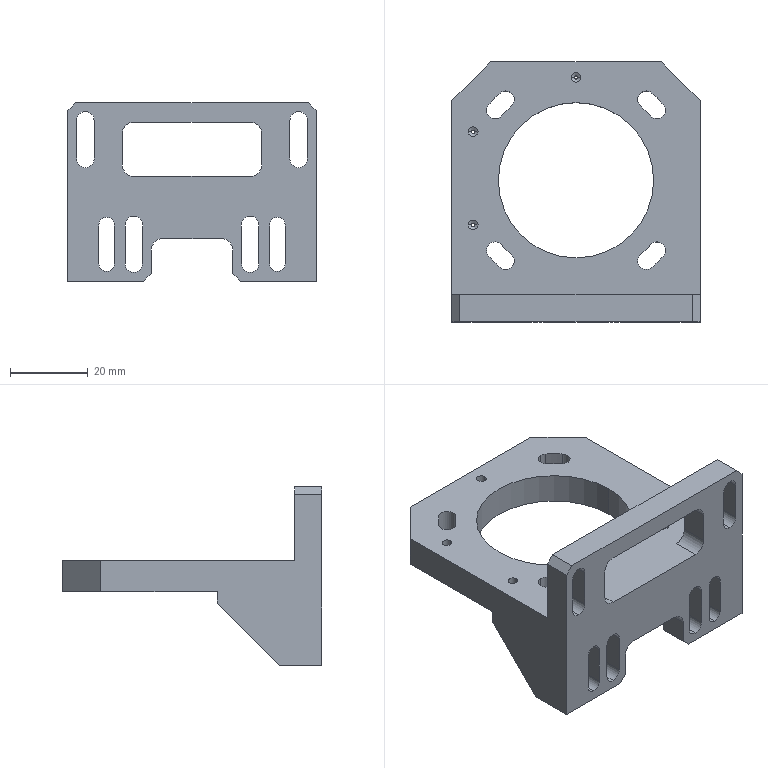NC program | NX | posted with a generic post | part box 64 x 67 x 46 mm
Lines 26761 to 27917 of 30645:
(ZLEVEL_PROFILE_COPY_2_COPY_COPY_COPY , TOOL : D6R0.5)
N53490 T05 M6
N53492 G54
N53494 G17 G0 G90 X-25.044 Y8.649 B0. C0. S7000 M3
N53496 G43 Z30. H5
N53498 Z0.929
N53500 G94 G1 Z-0.071 F1000.
N53502 X-25.504 Y9.429
N53504 G3 X-26.026 Y9.724 R0.6
N53506 G1 X-26.233 Y9.722 F3000.
N53508 X-33.751
N53510 X-33.974 Y9.724
N53512 X-33.975 Y9.687 Z-0.106
N53514 Y9.653 Z-0.141
N53516 X-33.751 Y9.651
N53518 X-26.233
N53520 X-26.025 Y9.653
N53522 X-26.024 Y9.616 Z-0.177
N53524 Y9.583 Z-0.212
N53526 X-26.5 Y9.581
N53528 X-33.5
N53530 X-33.976 Y9.582
N53532 X-33.977 Y9.545 Z-0.247
N53534 Y9.512 Z-0.283
N53536 X-33.5 Y9.51
N53538 X-26.5
N53540 X-26.022 Y9.512
N53542 Y9.475 Z-0.318
N53544 X-26.021 Y9.441 Z-0.354
N53546 X-26.5 Y9.439
N53548 X-33.5
N53550 X-33.979 Y9.441
N53552 Y9.404 Z-0.389
N53554 X-33.98 Y9.37 Z-0.424
N53556 X-33.5 Y9.369
N53558 X-26.5
N53560 X-26.02 Y9.37
N53562 Y9.333 Z-0.46
N53564 X-26.019 Y9.3 Z-0.495
N53566 X-26.5 Y9.298
N53568 X-33.5
N53570 X-33.981 Y9.299
N53572 Y9.263 Z-0.53
N53574 X-33.982 Y9.229 Z-0.566
N53576 X-33.5 Y9.227
N53578 X-26.5
N53580 X-26.018 Y9.229
N53582 X-26.017 Y9.192 Z-0.601
N53584 Y9.158 Z-0.636
N53586 X-26.5 Y9.156
N53588 X-33.5
N53590 X-33.983 Y9.158
N53592 X-33.984 Y9.121 Z-0.672
N53594 Y9.087 Z-0.707
N53596 X-33.5 Y9.086
N53598 X-26.5
N53600 X-26.016 Y9.087
N53602 X-26.015 Y9.05 Z-0.742
N53604 Y9.017 Z-0.778
N53606 X-26.5 Y9.015
N53608 X-33.5
N53610 X-33.985 Y9.016
N53612 X-33.986 Y8.98 Z-0.813
N53614 Y8.946 Z-0.849
N53616 X-33.5 Y8.944
N53618 X-26.5
N53620 X-26.014 Y8.946
N53622 X-26.013 Y8.909 Z-0.884
N53624 Y8.875 Z-0.919
N53626 X-26.5 Y8.874
N53628 X-33.5
N53630 X-33.987 Y8.875
N53632 X-33.988 Y8.838 Z-0.955
N53634 Y8.804 Z-0.99
N53636 X-33.5 Y8.803
N53638 X-26.5
N53640 X-26.012 Y8.805
N53642 X-26.011 Y8.768 Z-1.025
N53644 Y8.734 Z-1.061
N53646 X-26.5 Y8.732
N53648 X-33.5
N53650 X-33.989 Y8.734
N53652 Y8.697 Z-1.096
N53654 X-33.99 Y8.663 Z-1.131
N53656 X-33.5 Y8.662
N53658 X-26.5
N53660 X-26.01 Y8.663
N53662 Y8.626 Z-1.167
N53664 X-26.009 Y8.592 Z-1.202
N53666 X-26.5 Y8.591
N53668 X-33.5
N53670 X-33.991 Y8.592
N53672 Y8.555 Z-1.237
N53674 Y8.521 Z-1.273
N53676 X-33.5 Y8.52
N53678 X-26.5
N53680 X-26.008 Y8.522
N53682 Y8.485 Z-1.308
N53684 Y8.451 Z-1.344
N53686 X-26.5 Y8.449
N53688 X-33.5
N53690 X-33.992 Y8.451
N53692 X-33.993 Y8.414 Z-1.379
N53694 Y8.38 Z-1.414
N53696 X-33.5 Y8.379
N53698 X-26.5
N53700 X-26.007 Y8.38
N53702 X-26.006 Y8.343 Z-1.45
N53704 Y8.309 Z-1.485
N53706 X-26.5 Y8.308
N53708 X-33.5
N53710 X-33.994 Y8.309
N53712 Y8.273 Z-1.52
N53714 X-33.995 Y8.238 Z-1.556
N53716 X-33.5 Y8.237
N53718 X-26.5
N53720 X-26.005 Y8.239
N53722 Y8.202 Z-1.591
N53724 Y8.168 Z-1.626
N53726 X-26.5 Y8.167
N53728 X-33.5
N53730 X-33.995 Y8.168
N53732 X-33.996 Y8.131 Z-1.662
N53734 Y8.097 Z-1.697
N53736 X-33.5 Y8.096
N53738 X-26.5
N53740 X-26.004 Y8.097
N53742 Y8.06 Z-1.732
N53744 X-26.003 Y8.027 Z-1.768
N53746 X-26.5 Y8.025
N53748 X-33.5
N53750 X-33.997 Y8.026
N53752 Y7.99 Z-1.803
N53754 Y7.956 Z-1.838
N53756 X-33.5 Y7.954
N53758 X-26.5
N53760 X-26.003 Y7.956
N53762 X-26.002 Y7.919 Z-1.874
N53764 Y7.885 Z-1.909
N53766 X-26.5 Y7.884
N53768 X-33.5
N53770 X-33.998 Y7.885
N53772 Y7.848 Z-1.945
N53774 Y7.814 Z-1.98
N53776 X-33.5 Y7.813
N53778 X-26.5
N53780 X-26.002 Y7.814
N53782 X-26.001 Y7.778 Z-2.015
N53784 Y7.744 Z-2.051
N53786 X-26.5 Y7.742
N53788 X-33.5
N53790 X-33.999 Y7.743
N53792 Y7.707 Z-2.086
N53794 Y7.673 Z-2.121
N53796 X-33.5 Y7.672
N53798 X-26.5
N53800 X-26.001 Y7.673
N53802 Y7.639 Z-2.158
N53804 X-26. Y7.611 Z-2.195
N53806 X-26.489 Y7.609
N53808 X-26.511 Y7.603
N53810 X-33.49
N53812 X-33.502 Y7.609
N53814 X-34. Y7.61
N53816 Y7.582 Z-2.238
N53818 Y7.554 Z-2.281
N53820 X-33.515 Y7.553
N53822 X-33.499 Y7.551
N53824 X-26.5
N53826 X-26.488 Y7.553
N53828 X-26. Y7.555
N53830 Y7.533 Z-2.328
N53832 Y7.519 Z-2.375
N53834 X-26.488 Y7.518
N53836 X-26.5 Y7.516
N53838 X-33.5
N53840 X-33.515 Y7.518
N53842 X-34. Y7.519
N53844 Y7.509 Z-2.424
N53846 Y7.502 Z-2.474
N53848 X-33.5 Y7.501
N53850 X-26.488
N53852 X-26. Y7.502
N53854 X-25.999 Y7.501 Z-2.574
N53856 X-26.5 Y7.5
N53858 X-33.5
N53860 X-33.921
N53862 X-34. Y7.501
N53864 Z-2.674
N53866 X-33.921 Y7.5
N53868 X-33.5
N53870 X-26.5
N53872 X-26. Y7.501
N53874 Z-2.774
N53876 X-26.5 Y7.5
N53878 X-33.5
N53880 X-33.921
N53882 X-34.
N53884 Z-2.874
N53886 X-33.921
N53888 X-33.5
N53890 X-26.5
N53892 X-26. Y7.501
N53894 Z-2.974
N53896 X-26.5 Y7.5
N53898 X-33.5
N53900 X-33.921
N53902 X-34.
N53904 Z-3.074
N53906 X-33.921 Y7.499
N53908 X-33.5 Y7.5
N53910 X-26.5
N53912 X-26. Y7.501
N53914 Y7.5 Z-3.174
N53916 X-26.5
N53918 X-33.5
N53920 X-33.921 Y7.499
N53922 X-34. Y7.5
N53924 Z-3.274
N53926 X-33.921 Y7.499
N53928 X-33.5 Y7.5
N53930 X-26.5
N53932 X-26.
N53934 Z-3.374
N53936 X-26.5
N53938 X-33.5
N53940 X-33.921 Y7.499
N53942 X-34. Y7.5
N53944 Z-3.474
N53946 X-33.921 Y7.499
N53948 X-33.5 Y7.5
N53950 X-26.5
N53952 X-26.
N53954 Z-3.574
N53956 X-26.5
N53958 X-33.5
N53960 X-33.921 Y7.499
N53962 X-34. Y7.5
N53964 Z-3.674
N53966 X-33.921 Y7.499
N53968 X-33.5 Y7.5
N53970 X-26.5
N53972 X-26.
N53974 Z-3.774
N53976 X-26.5
N53978 X-33.5
N53980 X-33.921 Y7.499
N53982 X-34. Y7.5
N53984 Z-3.874
N53986 X-33.921 Y7.499
N53988 X-33.5 Y7.5
N53990 X-26.5
N53992 X-26.
N53994 Z-3.974
N53996 X-26.5
N53998 X-33.5
N54000 X-33.921 Y7.499
N54002 X-34. Y7.5
N54004 Z-4.074
N54006 X-33.921 Y7.499
N54008 X-33.5 Y7.5
N54010 X-26.5
N54012 X-26.
N54014 Z-4.174
N54016 X-26.5
N54018 X-33.5
N54020 X-33.921 Y7.499
N54022 X-34. Y7.5
N54024 Z-4.274
N54026 X-33.921 Y7.499
N54028 X-33.5 Y7.5
N54030 X-26.5
N54032 X-26.
N54034 Z-4.374
N54036 X-26.5
N54038 X-33.5
N54040 X-33.921 Y7.499
N54042 X-33.999 Y7.5
N54044 Z-4.474
N54046 X-33.921 Y7.499
N54048 X-33.5 Y7.5
N54050 X-26.5
N54052 X-26.
N54054 Z-4.574
N54056 X-26.5
N54058 X-33.5
N54060 X-33.921 Y7.499
N54062 X-33.999 Y7.5
N54064 Z-4.674
N54066 X-33.921 Y7.498
N54068 X-33.5 Y7.5
N54070 X-26.5
N54072 X-26.001
N54074 Z-4.774
N54076 X-26.5
N54078 X-33.5
N54080 X-33.921 Y7.498
N54082 X-33.999 Y7.5
N54084 Z-4.874
N54086 X-33.921 Y7.498
N54088 X-33.5 Y7.5
N54090 X-26.5
N54092 X-26.001
N54094 Z-4.974
N54096 X-26.5
N54098 X-33.5
N54100 X-33.921 Y7.498
N54102 X-33.999 Y7.499
N54104 Z-5.074
N54106 X-33.921 Y7.498
N54108 X-33.5 Y7.5
N54110 X-26.5
N54112 X-26.001
N54114 Z-5.174
N54116 X-26.5
N54118 X-33.5
N54120 X-33.921 Y7.498
N54122 X-33.999 Y7.499
N54124 Z-5.274
N54126 X-33.921 Y7.498
N54128 X-33.5 Y7.5
N54130 X-26.5
N54132 X-26.001
N54134 Z-5.374
N54136 X-26.5
N54138 X-33.5
N54140 X-33.921 Y7.498
N54142 X-33.999 Y7.499
N54144 Z-5.474
N54146 X-33.921 Y7.498
N54148 X-33.5 Y7.5
N54150 X-26.5
N54152 X-26.001
N54154 Z-5.574
N54156 X-26.5
N54158 X-33.5
N54160 X-33.921 Y7.498
N54162 X-33.998 Y7.499
N54164 Z-5.674
N54166 X-33.921 Y7.498
N54168 X-33.5 Y7.5
N54170 X-26.5
N54172 X-26.001
N54174 Z-5.774
N54176 X-26.5
N54178 X-33.5
N54180 X-33.921 Y7.498
N54182 X-33.998 Y7.499
N54184 Z-5.874
N54186 X-33.921 Y7.498
N54188 X-33.5 Y7.5
N54190 X-26.5
N54192 X-26.001
N54194 Z-5.974
N54196 X-26.5
N54198 X-33.5
N54200 X-33.921 Y7.498
N54202 X-33.998 Y7.499
N54204 Z-6.074
N54206 X-33.921 Y7.498
N54208 X-33.5 Y7.5
N54210 X-26.5
N54212 X-26.001
N54214 Z-6.174
N54216 X-26.5
N54218 X-33.5
N54220 X-33.921 Y7.498
N54222 X-33.998 Y7.499
N54224 Z-6.274
N54226 X-33.921 Y7.498
N54228 X-33.5 Y7.5
N54230 X-26.5
N54232 X-26.001
N54234 Z-6.374
N54236 X-26.5
N54238 X-33.5
N54240 X-33.921 Y7.497
N54242 X-33.998 Y7.499
N54244 X-33.997 Z-6.474
N54246 X-33.921 Y7.497
N54248 X-33.5 Y7.5
N54250 X-26.5
N54252 X-26.001
N54254 Z-6.574
N54256 X-26.5
N54258 X-33.5
N54260 X-33.921 Y7.497
N54262 X-33.997 Y7.499
N54264 Z-6.674
N54266 X-33.921 Y7.497
N54268 X-33.5 Y7.5
N54270 X-26.5
N54272 X-26.001
N54274 Z-6.774
N54276 X-26.5
N54278 X-33.5
N54280 X-33.921 Y7.497
N54282 X-33.997 Y7.499
N54284 Z-6.874
N54286 X-33.921 Y7.497
N54288 X-33.5 Y7.5
N54290 X-26.5
N54292 X-26.001
N54294 Z-6.974
N54296 X-26.5
N54298 X-33.5
N54300 X-33.921 Y7.497
N54302 X-33.997 Y7.499
N54304 Z-7.074
N54306 X-33.921 Y7.497
N54308 X-33.5 Y7.5
N54310 X-26.5
N54312 X-26.001
N54314 Z-7.174
N54316 X-26.5
N54318 X-33.5
N54320 X-33.921 Y7.497
N54322 X-33.997 Y7.498
N54324 X-33.996 Z-7.274
N54326 X-33.921 Y7.497
N54328 X-33.5 Y7.5
N54330 X-26.5
N54332 X-26.001
N54334 Z-7.374
N54336 X-26.5
N54338 X-33.5
N54340 X-33.921 Y7.497
N54342 X-33.996 Y7.498
N54344 Z-7.474
N54346 X-33.921 Y7.497
N54348 X-33.5 Y7.5
N54350 X-26.5
N54352 X-26.001
N54354 Z-7.574
N54356 X-26.5
N54358 X-33.5
N54360 X-33.921 Y7.497
N54362 X-33.996 Y7.498
N54364 Z-7.674
N54366 X-33.921 Y7.497
N54368 X-33.5 Y7.5
N54370 X-26.5
N54372 X-26.001
N54374 Z-7.774
N54376 X-26.5
N54378 X-33.5
N54380 X-33.921 Y7.497
N54382 X-33.996 Y7.498
N54384 Z-7.874
N54386 X-33.921 Y7.497
N54388 X-33.5 Y7.5
N54390 X-26.5
N54392 X-26.001
N54394 Y7.499 Z-7.974
N54396 X-26.5 Y7.5
N54398 X-33.5
N54400 X-33.921 Y7.496
N54402 X-33.995 Y7.498
N54404 Z-8.074
N54406 X-33.921 Y7.496
N54408 X-33.5 Y7.5
N54410 X-26.5
N54412 X-26.001 Y7.499
N54414 X-26.002 Z-8.174
N54416 X-26.5 Y7.5
N54418 X-33.5
N54420 X-33.921 Y7.496
N54422 X-33.995 Y7.498
N54424 Z-8.274
N54426 X-33.921 Y7.496
N54428 X-33.5 Y7.5
N54430 X-26.5
N54432 X-26.002 Y7.499
N54434 Z-8.374
N54436 X-26.5 Y7.5
N54438 X-33.5
N54440 X-33.995 Y7.498
N54442 Z-8.474
N54444 X-33.921 Y7.496
N54446 X-33.5 Y7.5
N54448 X-26.5
N54450 X-26.002 Y7.499
N54452 X-26.001 Y7.493 Z-8.574
N54454 X-26.575 Y7.494
N54456 X-26.608 Y7.499
N54458 X-33.584
N54460 X-33.609 Y7.502
N54462 X-33.625 Y7.495
N54464 X-33.999 Y7.49
N54466 Y7.479 Z-8.624
N54468 Y7.476 Z-8.674
N54470 G3 X-33.409 Y7.494 R8.389
N54472 G1 X-26.609
N54474 X-26.592 Y7.485
N54476 X-26.5 Y7.481
N54478 X-26.488 Y7.487
N54480 X-26.002 Y7.483
N54482 Y7.47 Z-8.723
N54484 Y7.465 Z-8.773
N54486 G2 X-26.646 Y7.485 R4.902
N54488 G1 X-33.409
N54490 X-33.501 Y7.473
N54492 X-33.999 Y7.458
N54494 Y7.446 Z-8.823
N54496 Y7.441 Z-8.872
N54498 X-33.517 Y7.45
N54500 X-33.501 Y7.459
N54502 X-33.409 Y7.472
N54504 X-26.611
N54506 G3 X-26.001 Y7.447 R3.499
N54508 G1 Y7.435 Z-8.922
N54510 Y7.423 Z-8.971
N54512 G2 X-26.73 Y7.455 R5.074
N54514 G1 X-33.317
N54516 G2 X-33.999 Y7.415 R4.455
N54518 G1 Y7.401 Z-9.02
N54520 Y7.388 Z-9.069
N54522 G3 X-33.294 Y7.434 R4.387
N54524 G1 X-26.753
N54526 G3 X-26. Y7.395 R4.721
N54528 G1 Y7.38 Z-9.117
N54530 Y7.365 Z-9.165
N54532 G2 X-26.733 Y7.41 R3.853
N54534 G1 X-33.292
N54536 G2 X-34. Y7.36 R3.818
N54538 G1 Y7.351 Z-9.213
N54540 Y7.331 Z-9.261
N54542 G3 X-33.311 Y7.381 R3.07
N54544 G1 X-26.695
N54546 G3 X-26. Y7.334 R2.954
N54548 G1 Y7.319 Z-9.308
N54550 Y7.302 Z-9.355
N54552 G2 X-26.738 Y7.349 R3.687
N54554 G1 X-33.255
N54556 G2 X-34. Y7.3 R4.005
N54558 G1 Y7.279 Z-9.402
N54560 Y7.261 Z-9.448
N54562 G3 X-33.242 Y7.313 R3.913
N54564 G1 X-26.763
N54566 G3 X-26. Y7.263 R3.811
N54568 G1 Y7.241 Z-9.494
N54570 Y7.225 Z-9.54
N54572 G2 X-26.766 Y7.274 R4.102
N54574 G1 X-33.249
N54576 G2 X-34. Y7.224 R3.862
N54578 G1 Y7.204 Z-9.584
N54580 Y7.174 Z-9.629
N54582 G3 X-33.278 Y7.23 R3.107
N54584 G1 X-26.721
N54586 G3 X-26. Y7.174 R3.027
N54588 G1 Y7.156 Z-9.673
N54590 Y7.125 Z-9.717
N54592 G2 X-26.756 Y7.184 R3.141
N54594 G1 X-33.245
N54596 G2 X-34. Y7.124 R3.171
N54598 G1 Y7.102 Z-9.76
N54600 Y7.076 Z-9.803
N54602 G3 X-33.235 Y7.134 R3.233
N54604 G1 X-26.767
N54606 G3 X-26. Y7.077 R3.223
N54608 G1 Y7.051 Z-9.844
N54610 Y7.022 Z-9.886
N54612 G2 X-26.777 Y7.081 R3.621
N54614 G1 X-33.224
N54616 G2 X-34. Y7.022 R3.685
N54618 G1 Y7. Z-9.927
N54620 Y6.961 Z-9.967
N54622 G3 X-33.23 Y7.024 R2.995
N54624 G1 X-26.774
N54626 G3 X-26. Y6.961 R2.996
N54628 G1 Y6.936 Z-10.007
N54630 Y6.902 Z-10.046
N54632 G2 X-26.801 Y6.965 R3.237
N54634 G1 X-33.2
N54636 G2 X-34. Y6.902 R3.273
N54638 G1 Y6.87 Z-10.084
N54640 Y6.838 Z-10.122
N54642 G3 X-33.188 Y6.902 R3.477
N54644 G1 X-26.813
N54646 G3 X-26. Y6.838 R3.432
N54648 G1 Y6.806 Z-10.159
N54650 Y6.772 Z-10.196
N54652 G2 X-26.817 Y6.837 R3.266
N54654 G1 X-33.184
N54656 G2 X-34. Y6.772 R3.293
N54658 G1 Y6.744 Z-10.231
N54660 Y6.708 Z-10.267
N54662 G3 X-33.18 Y6.769 R3.58
N54664 G1 X-26.821
N54666 G3 X-26. Y6.708 R3.542
N54668 G1 Y6.666 Z-10.301
N54670 Y6.629 Z-10.334
N54672 G2 X-26.825 Y6.698 R3.267
N54674 G1 X-33.162
N54676 G2 X-34. Y6.629 R3.51
N54678 G1 Y6.588 Z-10.367
N54680 Y6.553 Z-10.399
N54682 G3 X-33.157 Y6.626 R3.327
N54684 G1 X-26.829
N54686 G3 X-26. Y6.553 R3.115
N54688 G1 Y6.514 Z-10.43
N54690 Y6.472 Z-10.461
N54692 G2 X-26.834 Y6.551 R2.952
N54694 G1 X-33.167
N54696 G2 X-34. Y6.472 R2.984
N54698 G1 Y6.443 Z-10.49
N54700 Y6.393 Z-10.519
N54702 G3 X-33.154 Y6.474 R2.86
N54704 G1 X-26.844
N54706 G3 X-26. Y6.394 R2.814
N54708 G1 Y6.351 Z-10.546
N54710 Y6.31 Z-10.574
N54712 G2 X-26.887 Y6.396 R3.147
N54714 G1 X-33.113
N54716 G2 X-34. Y6.309 R3.18
N54718 G1 Y6.264 Z-10.6
N54720 Y6.225 Z-10.625
N54722 G3 X-33.091 Y6.316 R3.238
N54724 G1 X-26.897
N54726 G3 X-26. Y6.226 R3.069
N54728 G1 Y6.183 Z-10.649
N54730 Y6.132 Z-10.673
N54732 X-26.724 Y6.194
N54734 X-26.889 Y6.235
N54736 X-33.106
N54738 X-33.275 Y6.194
N54740 X-34. Y6.131
N54742 Y6.104 Z-10.696
N54744 Y6.035 Z-10.718
N54746 G3 X-33.087 Y6.154 R2.545
N54748 G1 X-26.897
N54750 X-26.745 Y6.097
N54752 X-26. Y6.035
N54754 Y6.001 Z-10.738
N54756 Y5.946 Z-10.759
N54758 X-26.804 Y6.017
N54760 X-26.961 Y6.072
N54762 X-33.034
N54764 G2 X-34. Y5.946 R2.758
N54766 G1 Y5.908 Z-10.777
N54768 Y5.866 Z-10.795
N54770 G3 X-33.021 Y5.99 R2.841
N54772 G1 X-26.989
N54774 G3 X-26. Y5.865 R2.913
N54776 G1 Y5.823 Z-10.812
N54778 Y5.763 Z-10.829
N54780 X-26.916 Y5.883
N54782 X-26.978 Y5.91
N54784 X-33.018
N54786 G2 X-34. Y5.769 R2.979
N54788 G1 Y5.748 Z-10.843
N54790 Y5.676 Z-10.858
N54792 G3 X-33.02 Y5.83 R2.254
N54794 G1 X-26.98
N54796 G3 X-26. Y5.665 R2.356
N54798 G1 Y5.636 Z-10.871
N54800 Y5.58 Z-10.884
N54802 X-26.916 Y5.7
N54804 X-27.026 Y5.753
N54806 X-32.973
N54808 G2 X-34. Y5.595 R2.305
N54810 G1 Y5.565 Z-10.895
N54812 Y5.526 Z-10.906
N54814 G3 X-32.944 Y5.68 R2.439
N54816 G1 X-27.054
N54818 X-26.916 Y5.619
N54820 X-26.003 Y5.505
N54822 X-26.065 Y5.422 Z-10.924
N54824 X-26.233 Y5.427
N54826 X-27.02 Y5.581
N54828 X-27.065 Y5.61
N54830 X-32.934
N54832 G2 X-33.999 Y5.458 R2.7
N54834 G1 Y5.396 Z-10.941
N54836 G3 X-32.96 Y5.541 R2.39
N54838 G1 X-27.027
N54840 X-26.916 Y5.491
N54842 X-26.119 Y5.349
N54844 X-26.163 Y5.289 Z-10.954
N54846 G2 X-27.003 Y5.477 R1.763
N54848 G1 X-33.023
N54850 G2 X-33.998 Y5.345 R2.122
N54852 G1 X-33.997 Y5.285 Z-10.965
N54854 G3 X-33.019 Y5.418 R2.198
N54856 G1 X-26.978
N54858 G3 X-26.199 Y5.241 R1.457
N54860 G1 X-26.228 Y5.201 Z-10.974
N54862 G2 X-26.954 Y5.362 R1.294
N54864 G1 X-33.026
N54866 G2 X-33.997 Y5.228 R2.054
N54868 G1 Y5.18 Z-10.981
N54870 G3 X-33.043 Y5.308 R1.948
N54872 G1 X-26.931
N54874 G3 X-26.424 Y5.175 R0.952
N54876 G1 X-26.492 Y5.147 Z-10.986
N54878 X-26.502 Y5.15
N54880 X-26.827 Y5.211
N54882 X-26.882 Y5.265
N54884 X-33.048
N54886 G2 X-33.911 Y5.136 R1.665
N54888 G1 X-33.779 Y5.076 Z-10.991
N54890 X-33.645 Y5.029 Z-10.995
N54892 X-33.516 Y5.009 Z-11.
N54894 X-33.072 Y5.112
N54896 X-26.723
N54898 X-26.504 Y5.043
N54900 Z-10.
N54902 G0 Z30.
N54904 X-34.956 Y-8.643
N54906 Z0.929
N54908 G1 Z-0.071 F1000.
N54910 X-34.496 Y-9.427
N54912 G3 X-33.974 Y-9.724 R0.6
N54914 G1 X-33.751 Y-9.722 F3000.
N54916 X-26.233
N54918 X-26.026 Y-9.724
N54920 X-26.025 Y-9.687 Z-0.106
N54922 Y-9.653 Z-0.141
N54924 X-26.233 Y-9.651
N54926 X-33.751
N54928 X-33.975 Y-9.653
N54930 X-33.976 Y-9.616 Z-0.177
N54932 X-33.977 Y-9.582 Z-0.212
N54934 X-33.5 Y-9.581
N54936 X-26.5
N54938 X-26.024 Y-9.583
N54940 X-26.023 Y-9.545 Z-0.247
N54942 X-26.022 Y-9.512 Z-0.283
N54944 X-26.5 Y-9.51
N54946 X-33.5
N54948 X-33.978 Y-9.512
N54950 Y-9.475 Z-0.318
N54952 X-33.979 Y-9.441 Z-0.354
N54954 X-33.5 Y-9.439
N54956 X-26.5
N54958 X-26.021 Y-9.441
N54960 Y-9.404 Z-0.389
N54962 X-26.02 Y-9.37 Z-0.424
N54964 X-26.5 Y-9.369
N54966 X-33.5
N54968 X-33.98 Y-9.37
N54970 X-33.981 Y-9.333 Z-0.46
N54972 Y-9.299 Z-0.495
N54974 X-33.5 Y-9.298
N54976 X-26.5
N54978 X-26.019 Y-9.3
N54980 Y-9.263 Z-0.53
N54982 X-26.018 Y-9.229 Z-0.566
N54984 X-26.5 Y-9.227
N54986 X-33.5
N54988 X-33.983 Y-9.229
N54990 Y-9.192 Z-0.601
N54992 X-33.984 Y-9.158 Z-0.636
N54994 X-33.5 Y-9.156
N54996 X-26.5
N54998 X-26.017 Y-9.158
N55000 X-26.016 Y-9.121 Z-0.672
N55002 Y-9.088 Z-0.707
N55004 X-26.5 Y-9.086
N55006 X-33.5
N55008 X-33.985 Y-9.087
N55010 Y-9.05 Z-0.742
N55012 X-33.986 Y-9.016 Z-0.778
N55014 X-33.5 Y-9.015
N55016 X-26.5
N55018 X-26.015 Y-9.017
N55020 X-26.014 Y-8.98 Z-0.813
N55022 Y-8.946 Z-0.849
N55024 X-26.5 Y-8.944
N55026 X-33.5
N55028 X-33.987 Y-8.946
N55030 X-33.988 Y-8.909 Z-0.884
N55032 Y-8.875 Z-0.919
N55034 X-33.5 Y-8.874
N55036 X-26.5
N55038 X-26.013 Y-8.875
N55040 X-26.012 Y-8.838 Z-0.955
N55042 Y-8.805 Z-0.99
N55044 X-26.5 Y-8.803
N55046 X-33.5
N55048 X-33.989 Y-8.804
N55050 X-33.99 Y-8.768 Z-1.025
N55052 Y-8.734 Z-1.061
N55054 X-33.5 Y-8.732
N55056 X-26.5
N55058 X-26.011 Y-8.734
N55060 Y-8.697 Z-1.096
N55062 X-26.01 Y-8.663 Z-1.131
N55064 X-26.5 Y-8.662
N55066 X-33.5
N55068 X-33.991 Y-8.663
N55070 Y-8.626 Z-1.167
N55072 X-33.992 Y-8.592 Z-1.202
N55074 X-33.5 Y-8.591
N55076 X-26.5
N55078 X-26.009 Y-8.592
N55080 Y-8.555 Z-1.237
N55082 X-26.008 Y-8.522 Z-1.273
N55084 X-26.5 Y-8.52
N55086 X-33.5
N55088 X-33.993 Y-8.521
N55090 Y-8.485 Z-1.308
N55092 X-33.994 Y-8.451 Z-1.344
N55094 X-33.5 Y-8.449
N55096 X-26.5
N55098 X-26.008 Y-8.451
N55100 X-26.007 Y-8.414 Z-1.379
N55102 Y-8.38 Z-1.414
N55104 X-26.5 Y-8.379
N55106 X-33.5
N55108 X-33.995 Y-8.38
N55110 Y-8.343 Z-1.45
N55112 Y-8.309 Z-1.485
N55114 X-33.5 Y-8.308
N55116 X-26.5
N55118 X-26.006 Y-8.31
N55120 Y-8.273 Z-1.52
N55122 X-26.005 Y-8.239 Z-1.556
N55124 X-26.5 Y-8.237
N55126 X-33.5
N55128 X-33.996 Y-8.238
N55130 X-33.997 Y-8.202 Z-1.591
N55132 Y-8.168 Z-1.626
N55134 X-33.5 Y-8.167
N55136 X-26.5
N55138 X-26.005 Y-8.168
N55140 X-26.004 Y-8.131 Z-1.662
N55142 Y-8.097 Z-1.697
N55144 X-26.5 Y-8.096
N55146 X-33.5
N55148 X-33.997 Y-8.097
N55150 X-33.998 Y-8.06 Z-1.732
N55152 Y-8.026 Z-1.768
N55154 X-33.5 Y-8.025
N55156 X-26.5
N55158 X-26.003 Y-8.027
N55160 Y-7.99 Z-1.803
N55162 Y-7.956 Z-1.838
N55164 X-26.5 Y-7.954
N55166 X-33.5
N55168 X-33.998 Y-7.956
N55170 X-33.999 Y-7.919 Z-1.874
N55172 Y-7.885 Z-1.909
N55174 X-33.5 Y-7.884
N55176 X-26.5
N55178 X-26.002 Y-7.885
N55180 Y-7.848 Z-1.945
N55182 Y-7.814 Z-1.98
N55184 X-26.5 Y-7.813
N55186 X-33.5
N55188 X-33.999 Y-7.814
N55190 Y-7.778 Z-2.015
N55192 Y-7.743 Z-2.051
N55194 X-33.5 Y-7.742
N55196 X-26.5
N55198 X-26.001 Y-7.744
N55200 Y-7.707 Z-2.086
N55202 Y-7.673 Z-2.121
N55204 X-26.5 Y-7.672
N55206 X-33.5
N55208 X-34. Y-7.673
N55210 Y-7.639 Z-2.158
N55212 Y-7.61 Z-2.195
N55214 X-33.505 Y-7.609
N55216 X-33.494 Y-7.603
N55218 X-26.518
N55220 X-26.499 Y-7.609
N55222 X-26. Y-7.611
N55224 Y-7.582 Z-2.238
N55226 Y-7.554 Z-2.281
N55228 X-26.062 Y-7.553
N55230 X-26.484
N55232 X-26.501 Y-7.551
N55234 X-33.5
N55236 X-33.52 Y-7.553
N55238 X-34. Y-7.554
N55240 Y-7.533 Z-2.328
N55242 Y-7.519 Z-2.375
N55244 X-33.52 Y-7.518
N55246 X-33.5 Y-7.516
N55248 X-26.5
N55250 X-26.484 Y-7.518
N55252 X-26.062
N55254 X-26. Y-7.519
N55256 X-25.999 Y-7.511 Z-2.424
N55258 Y-7.503 Z-2.474
N55260 X-26.062 Y-7.501
N55262 X-26.5
N55264 X-33.52
N55266 X-34. Y-7.503
N55268 Y-7.501 Z-2.574
N55270 X-33.5 Y-7.5
N55272 X-26.5
N55274 X-26.062 Y-7.498
N55276 X-25.998 Y-7.5
N55278 Z-2.674
N55280 X-26.062 Y-7.498
N55282 X-26.5 Y-7.5
N55284 X-33.5
N55286 X-34. Y-7.501
N55288 Z-2.774
N55290 X-33.5 Y-7.5
N55292 X-26.5
N55294 X-26.062 Y-7.498
N55296 X-25.999 Y-7.5
N55298 Z-2.874
N55300 X-26.062 Y-7.498
N55302 X-26.5 Y-7.5
N55304 X-33.5
N55306 X-34. Y-7.501
N55308 Z-2.974
N55310 X-33.5 Y-7.5
N55312 X-26.5
N55314 X-26.062 Y-7.498
N55316 X-25.999 Y-7.5
N55318 Z-3.074
N55320 X-26.062 Y-7.498
N55322 X-26.5 Y-7.5
N55324 X-33.5
N55326 X-34. Y-7.501
N55328 Z-3.174
N55330 X-33.5 Y-7.5
N55332 X-26.5
N55334 X-26.062 Y-7.498
N55336 X-25.999 Y-7.5
N55338 Z-3.274
N55340 X-26.062 Y-7.498
N55342 X-26.5 Y-7.5
N55344 X-33.5
N55346 X-34. Y-7.501
N55348 Z-3.374
N55350 X-33.5 Y-7.5
N55352 X-26.5
N55354 X-26.062 Y-7.498
N55356 X-26. Y-7.5
N55358 Z-3.474
N55360 X-26.062 Y-7.498
N55362 X-26.5 Y-7.5
N55364 X-33.5
N55366 X-34. Y-7.501
N55368 Z-3.574
N55370 X-33.5 Y-7.5
N55372 X-26.5
N55374 X-26.062 Y-7.498
N55376 X-26. Y-7.5
N55378 Z-3.674
N55380 X-26.062 Y-7.498
N55382 X-26.5 Y-7.5
N55384 X-33.5
N55386 X-34. Y-7.501
N55388 Z-3.774
N55390 X-33.5 Y-7.5
N55392 X-26.5
N55394 X-26.062 Y-7.497
N55396 X-26. Y-7.5
N55398 Z-3.874
N55400 X-26.062 Y-7.497
N55402 X-26.5 Y-7.5
N55404 X-33.5
N55406 X-34. Y-7.501
N55408 Z-3.974
N55410 X-33.5 Y-7.5
N55412 X-26.5
N55414 X-26.062 Y-7.497
N55416 X-26. Y-7.499
N55418 X-26.001 Z-4.074
N55420 X-26.062 Y-7.497
N55422 X-26.5 Y-7.5
N55424 X-33.5
N55426 X-34. Y-7.501
N55428 Z-4.174
N55430 X-33.5 Y-7.5
N55432 X-26.5
N55434 X-26.062 Y-7.497
N55436 X-26.001 Y-7.499
N55438 Z-4.274
N55440 X-26.062 Y-7.497
N55442 X-26.5 Y-7.5
N55444 X-33.5
N55446 X-34. Y-7.501
N55448 Z-4.374
N55450 X-33.5 Y-7.5
N55452 X-26.5
N55454 X-26.062 Y-7.497
N55456 X-26.001 Y-7.499
N55458 Z-4.474
N55460 X-26.062 Y-7.497
N55462 X-26.5 Y-7.5
N55464 X-33.5
N55466 X-34. Y-7.501
N55468 Z-4.574
N55470 X-33.5 Y-7.5
N55472 X-26.5
N55474 X-26.062 Y-7.497
N55476 X-26.001 Y-7.499
N55478 X-26.002 Z-4.674
N55480 X-26.062 Y-7.497
N55482 X-26.5 Y-7.5
N55484 X-33.5
N55486 X-34. Y-7.501
N55488 Z-4.774
N55490 X-33.5 Y-7.5
N55492 X-26.5
N55494 X-26.062 Y-7.497
N55496 X-26.002 Y-7.499
N55498 Z-4.874
N55500 X-26.062 Y-7.497
N55502 X-26.5 Y-7.5
N55504 X-33.5
N55506 X-34. Y-7.501
N55508 Z-4.974
N55510 X-33.5 Y-7.5
N55512 X-26.5
N55514 X-26.062 Y-7.497
N55516 X-26.002 Y-7.499
N55518 Z-5.074
N55520 X-26.062 Y-7.497
N55522 X-26.5 Y-7.5
N55524 X-33.5
N55526 X-34. Y-7.501
N55528 Z-5.174
N55530 X-33.5 Y-7.5
N55532 X-26.5
N55534 X-26.062 Y-7.497
N55536 X-26.002 Y-7.499
N55538 Z-5.274
N55540 X-26.062 Y-7.497
N55542 X-26.5 Y-7.5
N55544 X-33.5
N55546 X-34. Y-7.501
N55548 Z-5.374
N55550 X-33.5 Y-7.5
N55552 X-26.5
N55554 X-26.062 Y-7.497
N55556 X-26.003 Y-7.499
N55558 Z-5.474
N55560 X-26.062 Y-7.497
N55562 X-26.5 Y-7.5
N55564 X-33.5
N55566 X-34. Y-7.501
N55568 Z-5.574
N55570 X-33.5 Y-7.5
N55572 X-26.5
N55574 X-26.062 Y-7.497
N55576 X-26.003 Y-7.499
N55578 Z-5.674
N55580 X-26.062 Y-7.497
N55582 X-26.5 Y-7.5
N55584 X-33.5
N55586 X-34. Y-7.501
N55588 Y-7.5 Z-5.774
N55590 X-33.5
N55592 X-26.5
N55594 X-26.062 Y-7.497
N55596 X-26.003 Y-7.499
N55598 Z-5.874
N55600 X-26.062 Y-7.497
N55602 X-26.5 Y-7.5
N55604 X-33.5
N55606 X-34.
N55608 Z-5.974
N55610 X-33.5
N55612 X-26.5
N55614 X-26.062 Y-7.497
N55616 X-26.003 Y-7.499
N55618 X-26.004 Z-6.074
N55620 X-26.062 Y-7.497
N55622 X-26.5 Y-7.5
N55624 X-33.5
N55626 X-34.
N55628 Z-6.174
N55630 X-33.5
N55632 X-26.5
N55634 X-26.062 Y-7.497
N55636 X-26.004 Y-7.499
N55638 Z-6.274
N55640 X-26.062 Y-7.497
N55642 X-26.5 Y-7.5
N55644 X-33.5
N55646 X-34.
N55648 Z-6.374
N55650 X-33.5
N55652 X-26.5
N55654 X-26.062 Y-7.497
N55656 X-26.004 Y-7.499
N55658 Z-6.474
N55660 X-26.062 Y-7.497
N55662 X-26.5 Y-7.5
N55664 X-33.5
N55666 X-34.
N55668 Z-6.574
N55670 X-33.5
N55672 X-26.5
N55674 X-26.062 Y-7.497
N55676 X-26.004 Y-7.499
N55678 X-26.005 Y-7.498 Z-6.674
N55680 X-26.062 Y-7.497
N55682 X-26.5 Y-7.5
N55684 X-33.5
N55686 X-34.
N55688 Z-6.774
N55690 X-33.5
N55692 X-26.5
N55694 X-26.062 Y-7.497
N55696 X-26.005 Y-7.498
N55698 Z-6.874
N55700 X-26.062 Y-7.497
N55702 X-26.5 Y-7.5
N55704 X-33.5
N55706 X-34.
N55708 Z-6.974
N55710 X-33.5
N55712 X-26.5
N55714 X-26.062 Y-7.497
N55716 X-26.005 Y-7.498
N55718 Z-7.074
N55720 X-26.062 Y-7.497
N55722 X-26.5 Y-7.5
N55724 X-33.5
N55726 X-34.
N55728 Z-7.174
N55730 X-33.5
N55732 X-26.5
N55734 X-26.062 Y-7.496
N55736 X-26.005 Y-7.498
N55738 Z-7.274
N55740 X-26.062 Y-7.496
N55742 X-26.5 Y-7.5
N55744 X-33.5
N55746 X-34.
N55748 Z-7.374
N55750 X-33.5
N55752 X-26.5
N55754 X-26.062 Y-7.496
N55756 X-26.005 Y-7.498
N55758 X-26.006 Z-7.474
N55760 X-26.062 Y-7.496
N55762 X-26.5 Y-7.5
N55764 X-33.5
N55766 X-34.
N55768 Z-7.574
N55770 X-33.5
N55772 X-26.5
N55774 X-26.062 Y-7.496
N55776 X-26.006 Y-7.498
N55778 Z-7.674
N55780 X-26.062 Y-7.496
N55782 X-26.5 Y-7.5
N55784 X-33.5
N55786 X-34.
N55788 Z-7.774
N55790 X-33.5
N55792 X-26.5
N55794 X-26.062 Y-7.496
N55796 X-26.006 Y-7.498